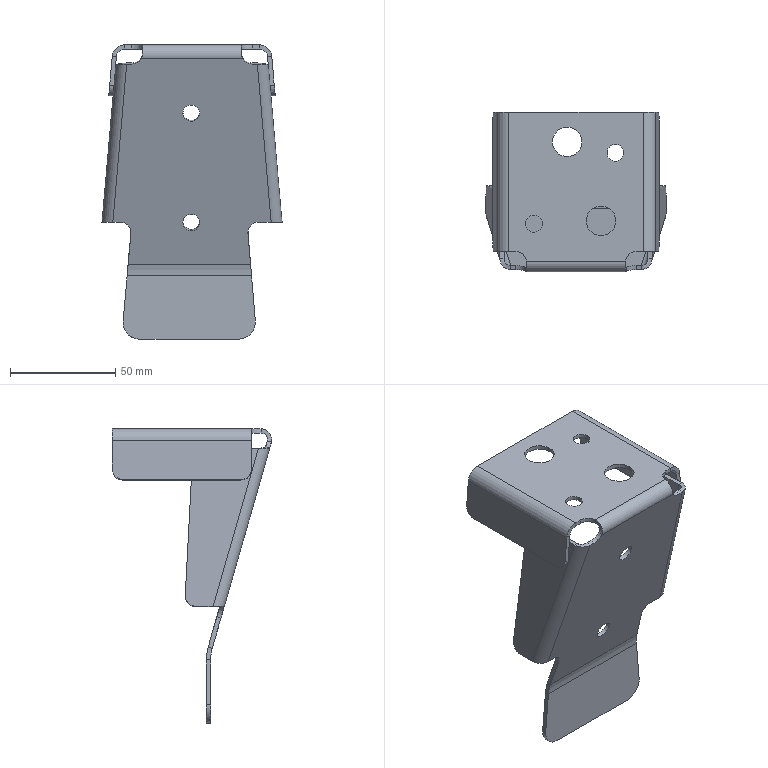Part | 1 solid | 90 faces | box 85.394 x 75.619 x 139.609 mm | volume 41726 mm3 | plane 30 | spline 28 | cylinder 26 | other 6 | commonest cylinder face diameters 8 x10 14 x4 6 x3 10 x3 12 x2 16 x2